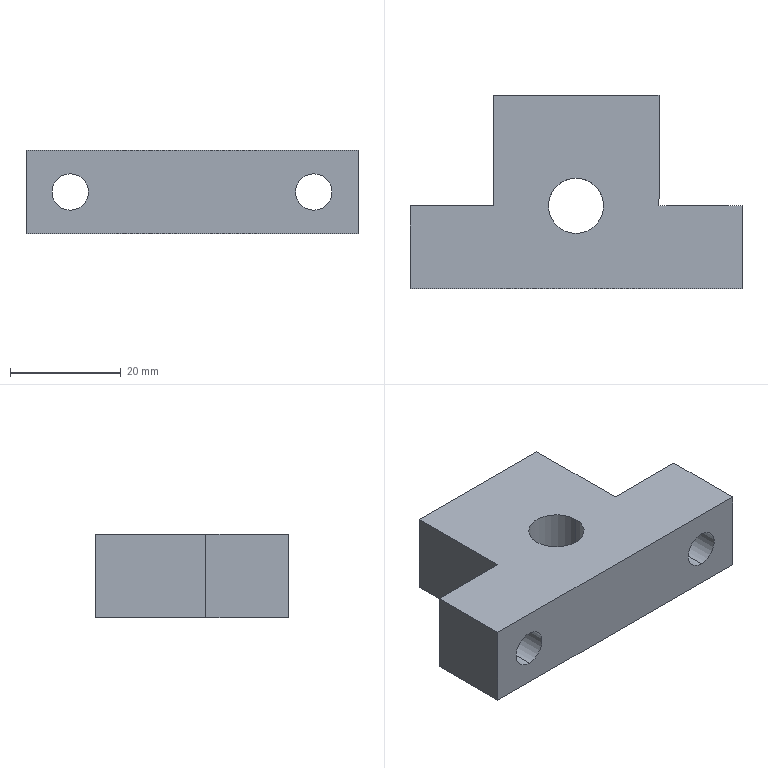Part | SolidWorks | features 3DProfileFeature 1, Extrusion 1, HoleWzd 1, ICE 1 | 1 solid | 22 faces | box 60 x 35 x 15 mm | volume 19468 mm3 | plane 12 | cylinder 10 | commonest cylinder face diameters 6.6 x4 11 x4 10 x2
STEP:
#1=CARTESIAN_POINT('',(8.,8.2,2.));
#2=VERTEX_POINT('',#1);
#3=CARTESIAN_POINT('',(8.,8.2,13.));
#4=VERTEX_POINT('',#3);
#5=CARTESIAN_POINT('',(8.,8.2,7.5));
#6=DIRECTION('',(0.,1.,0.));
#7=DIRECTION('',(0.,0.,1.));
#8=AXIS2_PLACEMENT_3D('',#5,#6,#7);
#9=CIRCLE('',#8,5.5);
#10=EDGE_CURVE('',#2,#4,#9,.T.);
#11=ORIENTED_EDGE('',*,*,#10,.F.);
#12=CARTESIAN_POINT('',(8.,15.,2.));
#13=VERTEX_POINT('',#12);
#14=CARTESIAN_POINT('',(8.,15.,2.));
#15=DIRECTION('',(0.,1.,0.));
#16=VECTOR('',#15,1000.);
#17=LINE('',#14,#16);
#18=EDGE_CURVE('',#2,#13,#17,.T.);
#19=ORIENTED_EDGE('',*,*,#18,.T.);
#20=CARTESIAN_POINT('',(8.,15.,13.));
#21=VERTEX_POINT('',#20);
#22=CARTESIAN_POINT('',(8.,15.,7.5));
#23=DIRECTION('',(0.,1.,0.));
#24=DIRECTION('',(0.,0.,1.));
#25=AXIS2_PLACEMENT_3D('',#22,#23,#24);
#26=CIRCLE('',#25,5.5);
#27=EDGE_CURVE('',#13,#21,#26,.T.);
#28=ORIENTED_EDGE('',*,*,#27,.T.);
#29=CARTESIAN_POINT('',(8.,15.,13.));
#30=DIRECTION('',(0.,1.,0.));
#31=VECTOR('',#30,1000.);
#32=LINE('',#29,#31);
#33=EDGE_CURVE('',#4,#21,#32,.T.);
#34=ORIENTED_EDGE('',*,*,#33,.F.);
#35=EDGE_LOOP('',(#11,#19,#28,#34));
#36=FACE_OUTER_BOUND('',#35,.T.);
#37=CARTESIAN_POINT('',(8.,15.,7.5));
#38=DIRECTION('',(0.,1.,0.));
#39=DIRECTION('',(0.,0.,1.));
#40=AXIS2_PLACEMENT_3D('',#37,#38,#39);
#41=CYLINDRICAL_SURFACE('',#40,5.5);
#42=ADVANCED_FACE('',(#36),#41,.F.);
#43=CARTESIAN_POINT('',(8.,0.,4.2));
#44=VERTEX_POINT('',#43);
#45=CARTESIAN_POINT('',(8.,0.,10.8));
#46=VERTEX_POINT('',#45);
#47=CARTESIAN_POINT('',(8.,0.,7.5));
#48=DIRECTION('',(0.,1.,0.));
#49=DIRECTION('',(0.,0.,1.));
#50=AXIS2_PLACEMENT_3D('',#47,#48,#49);
#51=CIRCLE('',#50,3.3);
#52=EDGE_CURVE('',#44,#46,#51,.T.);
#53=ORIENTED_EDGE('',*,*,#52,.F.);
#54=CARTESIAN_POINT('',(8.,8.2,4.2));
#55=VERTEX_POINT('',#54);
#56=CARTESIAN_POINT('',(8.,15.,4.2));
#57=DIRECTION('',(0.,1.,0.));
#58=VECTOR('',#57,1000.);
#59=LINE('',#56,#58);
#60=EDGE_CURVE('',#44,#55,#59,.T.);
#61=ORIENTED_EDGE('',*,*,#60,.T.);
#62=CARTESIAN_POINT('',(8.,8.2,10.8));
#63=VERTEX_POINT('',#62);
#64=CARTESIAN_POINT('',(8.,8.2,7.5));
#65=DIRECTION('',(0.,1.,0.));
#66=DIRECTION('',(0.,0.,1.));
#67=AXIS2_PLACEMENT_3D('',#64,#65,#66);
#68=CIRCLE('',#67,3.3);
#69=EDGE_CURVE('',#55,#63,#68,.T.);
#70=ORIENTED_EDGE('',*,*,#69,.T.);
#71=CARTESIAN_POINT('',(8.,15.,10.8));
#72=DIRECTION('',(0.,1.,0.));
#73=VECTOR('',#72,1000.);
#74=LINE('',#71,#73);
#75=EDGE_CURVE('',#46,#63,#74,.T.);
#76=ORIENTED_EDGE('',*,*,#75,.F.);
#77=EDGE_LOOP('',(#53,#61,#70,#76));
#78=FACE_OUTER_BOUND('',#77,.T.);
#79=CARTESIAN_POINT('',(8.,15.,7.5));
#80=DIRECTION('',(0.,1.,0.));
#81=DIRECTION('',(0.,0.,1.));
#82=AXIS2_PLACEMENT_3D('',#79,#80,#81);
#83=CYLINDRICAL_SURFACE('',#82,3.3);
#84=ADVANCED_FACE('',(#78),#83,.F.);
#85=CARTESIAN_POINT('',(52.,8.2,2.));
#86=VERTEX_POINT('',#85);
#87=CARTESIAN_POINT('',(52.,8.2,13.));
#88=VERTEX_POINT('',#87);
#89=CARTESIAN_POINT('',(52.,8.2,7.5));
#90=DIRECTION('',(0.,1.,0.));
#91=DIRECTION('',(0.,0.,1.));
#92=AXIS2_PLACEMENT_3D('',#89,#90,#91);
#93=CIRCLE('',#92,5.5);
#94=EDGE_CURVE('',#86,#88,#93,.T.);
#95=ORIENTED_EDGE('',*,*,#94,.F.);
#96=CARTESIAN_POINT('',(52.,15.,2.));
#97=VERTEX_POINT('',#96);
#98=CARTESIAN_POINT('',(52.,15.,2.));
#99=DIRECTION('',(0.,1.,0.));
#100=VECTOR('',#99,1000.);
#101=LINE('',#98,#100);
#102=EDGE_CURVE('',#86,#97,#101,.T.);
#103=ORIENTED_EDGE('',*,*,#102,.T.);
#104=CARTESIAN_POINT('',(52.,15.,13.));
#105=VERTEX_POINT('',#104);
#106=CARTESIAN_POINT('',(52.,15.,7.5));
#107=DIRECTION('',(0.,1.,0.));
#108=DIRECTION('',(0.,0.,1.));
#109=AXIS2_PLACEMENT_3D('',#106,#107,#108);
#110=CIRCLE('',#109,5.5);
#111=EDGE_CURVE('',#97,#105,#110,.T.);
#112=ORIENTED_EDGE('',*,*,#111,.T.);
#113=CARTESIAN_POINT('',(52.,15.,13.));
#114=DIRECTION('',(0.,1.,0.));
#115=VECTOR('',#114,1000.);
#116=LINE('',#113,#115);
#117=EDGE_CURVE('',#88,#105,#116,.T.);
#118=ORIENTED_EDGE('',*,*,#117,.F.);
#119=EDGE_LOOP('',(#95,#103,#112,#118));
#120=FACE_OUTER_BOUND('',#119,.T.);
#121=CARTESIAN_POINT('',(52.,15.,7.5));
#122=DIRECTION('',(0.,1.,0.));
#123=DIRECTION('',(0.,0.,1.));
#124=AXIS2_PLACEMENT_3D('',#121,#122,#123);
#125=CYLINDRICAL_SURFACE('',#124,5.5);
#126=ADVANCED_FACE('',(#120),#125,.F.);
#127=CARTESIAN_POINT('',(52.,0.,4.2));
#128=VERTEX_POINT('',#127);
#129=CARTESIAN_POINT('',(52.,0.,10.8));
#130=VERTEX_POINT('',#129);
#131=CARTESIAN_POINT('',(52.,0.,7.5));
#132=DIRECTION('',(0.,1.,0.));
#133=DIRECTION('',(0.,0.,1.));
#134=AXIS2_PLACEMENT_3D('',#131,#132,#133);
#135=CIRCLE('',#134,3.3);
#136=EDGE_CURVE('',#128,#130,#135,.T.);
#137=ORIENTED_EDGE('',*,*,#136,.F.);
#138=CARTESIAN_POINT('',(52.,8.2,4.2));
#139=VERTEX_POINT('',#138);
#140=CARTESIAN_POINT('',(52.,15.,4.2));
#141=DIRECTION('',(0.,1.,0.));
#142=VECTOR('',#141,1000.);
#143=LINE('',#140,#142);
#144=EDGE_CURVE('',#128,#139,#143,.T.);
#145=ORIENTED_EDGE('',*,*,#144,.T.);
#146=CARTESIAN_POINT('',(52.,8.2,10.8));
#147=VERTEX_POINT('',#146);
#148=CARTESIAN_POINT('',(52.,8.2,7.5));
#149=DIRECTION('',(0.,1.,0.));
#150=DIRECTION('',(0.,0.,1.));
#151=AXIS2_PLACEMENT_3D('',#148,#149,#150);
#152=CIRCLE('',#151,3.3);
#153=EDGE_CURVE('',#139,#147,#152,.T.);
#154=ORIENTED_EDGE('',*,*,#153,.T.);
#155=CARTESIAN_POINT('',(52.,15.,10.8));
#156=DIRECTION('',(0.,1.,0.));
#157=VECTOR('',#156,1000.);
#158=LINE('',#155,#157);
#159=EDGE_CURVE('',#130,#147,#158,.T.);
#160=ORIENTED_EDGE('',*,*,#159,.F.);
#161=EDGE_LOOP('',(#137,#145,#154,#160));
#162=FACE_OUTER_BOUND('',#161,.T.);
#163=CARTESIAN_POINT('',(52.,15.,7.5));
#164=DIRECTION('',(0.,1.,0.));
#165=DIRECTION('',(0.,0.,1.));
#166=AXIS2_PLACEMENT_3D('',#163,#164,#165);
#167=CYLINDRICAL_SURFACE('',#166,3.3);
#168=ADVANCED_FACE('',(#162),#167,.F.);
#169=CARTESIAN_POINT('',(25.,15.,0.));
#170=VERTEX_POINT('',#169);
#171=CARTESIAN_POINT('',(35.,15.,0.));
#172=VERTEX_POINT('',#171);
#173=CARTESIAN_POINT('',(30.,15.,0.));
#174=DIRECTION('',(0.,0.,1.));
#175=DIRECTION('',(1.,0.,0.));
#176=AXIS2_PLACEMENT_3D('',#173,#174,#175);
#177=CIRCLE('',#176,5.);
#178=EDGE_CURVE('',#170,#172,#177,.T.);
#179=ORIENTED_EDGE('',*,*,#178,.F.);
#180=CARTESIAN_POINT('',(25.,15.,15.));
#181=VERTEX_POINT('',#180);
#182=CARTESIAN_POINT('',(25.,15.,0.));
#183=DIRECTION('',(0.,0.,1.));
#184=VECTOR('',#183,1000.);
#185=LINE('',#182,#184);
#186=EDGE_CURVE('',#170,#181,#185,.T.);
#187=ORIENTED_EDGE('',*,*,#186,.T.);
#188=CARTESIAN_POINT('',(35.,15.,15.));
#189=VERTEX_POINT('',#188);
#190=CARTESIAN_POINT('',(30.,15.,15.));
#191=DIRECTION('',(0.,0.,1.));
#192=DIRECTION('',(1.,0.,0.));
#193=AXIS2_PLACEMENT_3D('',#190,#191,#192);
#194=CIRCLE('',#193,5.);
#195=EDGE_CURVE('',#181,#189,#194,.T.);
#196=ORIENTED_EDGE('',*,*,#195,.T.);
#197=CARTESIAN_POINT('',(35.,15.,0.));
#198=DIRECTION('',(0.,0.,1.));
#199=VECTOR('',#198,1000.);
#200=LINE('',#197,#199);
#201=EDGE_CURVE('',#172,#189,#200,.T.);
#202=ORIENTED_EDGE('',*,*,#201,.F.);
#203=EDGE_LOOP('',(#179,#187,#196,#202));
#204=FACE_OUTER_BOUND('',#203,.T.);
#205=CARTESIAN_POINT('',(30.,15.,0.));
#206=DIRECTION('',(0.,0.,1.));
#207=DIRECTION('',(1.,0.,0.));
#208=AXIS2_PLACEMENT_3D('',#205,#206,#207);
#209=CYLINDRICAL_SURFACE('',#208,5.);
#210=ADVANCED_FACE('',(#204),#209,.F.);
#211=CARTESIAN_POINT('',(8.,0.,7.5));
#212=DIRECTION('',(0.,1.,0.));
#213=DIRECTION('',(0.,0.,1.));
#214=AXIS2_PLACEMENT_3D('',#211,#212,#213);
#215=CIRCLE('',#214,3.3);
#216=EDGE_CURVE('',#46,#44,#215,.T.);
#217=ORIENTED_EDGE('',*,*,#216,.T.);
#218=ORIENTED_EDGE('',*,*,#52,.T.);
#219=EDGE_LOOP('',(#217,#218));
#220=FACE_BOUND('',#219,.T.);
#221=CARTESIAN_POINT('',(52.,0.,7.5));
#222=DIRECTION('',(0.,1.,0.));
#223=DIRECTION('',(0.,0.,1.));
#224=AXIS2_PLACEMENT_3D('',#221,#222,#223);
#225=CIRCLE('',#224,3.3);
#226=EDGE_CURVE('',#130,#128,#225,.T.);
#227=ORIENTED_EDGE('',*,*,#226,.T.);
#228=ORIENTED_EDGE('',*,*,#136,.T.);
#229=EDGE_LOOP('',(#227,#228));
#230=FACE_BOUND('',#229,.T.);
#231=CARTESIAN_POINT('',(0.,0.,0.));
#232=VERTEX_POINT('',#231);
#233=CARTESIAN_POINT('',(60.,0.,0.));
#234=VERTEX_POINT('',#233);
#235=CARTESIAN_POINT('',(60.,0.,0.));
#236=DIRECTION('',(1.,0.,0.));
#237=VECTOR('',#236,1000.);
#238=LINE('',#235,#237);
#239=EDGE_CURVE('',#232,#234,#238,.T.);
#240=ORIENTED_EDGE('',*,*,#239,.T.);
#241=CARTESIAN_POINT('',(60.,0.,15.));
#242=VERTEX_POINT('',#241);
#243=CARTESIAN_POINT('',(60.,0.,15.));
#244=DIRECTION('',(0.,0.,-1.));
#245=VECTOR('',#244,1000.);
#246=LINE('',#243,#245);
#247=EDGE_CURVE('',#242,#234,#246,.T.);
#248=ORIENTED_EDGE('',*,*,#247,.F.);
#249=CARTESIAN_POINT('',(0.,0.,15.));
#250=VERTEX_POINT('',#249);
#251=CARTESIAN_POINT('',(60.,0.,15.));
#252=DIRECTION('',(1.,0.,0.));
#253=VECTOR('',#252,1000.);
#254=LINE('',#251,#253);
#255=EDGE_CURVE('',#250,#242,#254,.T.);
#256=ORIENTED_EDGE('',*,*,#255,.F.);
#257=CARTESIAN_POINT('',(0.,0.,15.));
#258=DIRECTION('',(0.,0.,-1.));
#259=VECTOR('',#258,1000.);
#260=LINE('',#257,#259);
#261=EDGE_CURVE('',#250,#232,#260,.T.);
#262=ORIENTED_EDGE('',*,*,#261,.T.);
#263=EDGE_LOOP('',(#240,#248,#256,#262));
#264=FACE_OUTER_BOUND('',#263,.T.);
#265=CARTESIAN_POINT('',(60.,0.,15.));
#266=DIRECTION('',(0.,1.,0.));
#267=DIRECTION('',(-1.,0.,0.));
#268=AXIS2_PLACEMENT_3D('',#265,#266,#267);
#269=PLANE('',#268);
#270=ADVANCED_FACE('',(#220,#230,#264),#269,.F.);
#271=CARTESIAN_POINT('',(60.,15.,0.));
#272=VERTEX_POINT('',#271);
#273=CARTESIAN_POINT('',(60.,0.,0.));
#274=DIRECTION('',(0.,1.,0.));
#275=VECTOR('',#274,1000.);
#276=LINE('',#273,#275);
#277=EDGE_CURVE('',#234,#272,#276,.T.);
#278=ORIENTED_EDGE('',*,*,#277,.T.);
#279=CARTESIAN_POINT('',(60.,15.,15.));
#280=VERTEX_POINT('',#279);
#281=CARTESIAN_POINT('',(60.,15.,15.));
#282=DIRECTION('',(0.,0.,-1.));
#283=VECTOR('',#282,1000.);
#284=LINE('',#281,#283);
#285=EDGE_CURVE('',#280,#272,#284,.T.);
#286=ORIENTED_EDGE('',*,*,#285,.F.);
#287=CARTESIAN_POINT('',(60.,0.,15.));
#288=DIRECTION('',(0.,1.,0.));
#289=VECTOR('',#288,1000.);
#290=LINE('',#287,#289);
#291=EDGE_CURVE('',#242,#280,#290,.T.);
#292=ORIENTED_EDGE('',*,*,#291,.F.);
#293=ORIENTED_EDGE('',*,*,#247,.T.);
#294=EDGE_LOOP('',(#278,#286,#292,#293));
#295=FACE_OUTER_BOUND('',#294,.T.);
#296=CARTESIAN_POINT('',(60.,0.,15.));
#297=DIRECTION('',(-1.,0.,0.));
#298=DIRECTION('',(0.,0.,1.));
#299=AXIS2_PLACEMENT_3D('',#296,#297,#298);
#300=PLANE('',#299);
#301=ADVANCED_FACE('',(#295),#300,.F.);
#302=CARTESIAN_POINT('',(52.,15.,7.5));
#303=DIRECTION('',(0.,1.,0.));
#304=DIRECTION('',(0.,0.,1.));
#305=AXIS2_PLACEMENT_3D('',#302,#303,#304);
#306=CIRCLE('',#305,5.5);
#307=EDGE_CURVE('',#105,#97,#306,.T.);
#308=ORIENTED_EDGE('',*,*,#307,.F.);
#309=ORIENTED_EDGE('',*,*,#111,.F.);
#310=EDGE_LOOP('',(#308,#309));
#311=FACE_BOUND('',#310,.T.);
#312=CARTESIAN_POINT('',(45.,15.,0.));
#313=VERTEX_POINT('',#312);
#314=CARTESIAN_POINT('',(60.,15.,0.));
#315=DIRECTION('',(-1.,0.,0.));
#316=VECTOR('',#315,1000.);
#317=LINE('',#314,#316);
#318=EDGE_CURVE('',#272,#313,#317,.T.);
#319=ORIENTED_EDGE('',*,*,#318,.T.);
#320=CARTESIAN_POINT('',(45.,15.,15.));
#321=VERTEX_POINT('',#320);
#322=CARTESIAN_POINT('',(45.,15.,15.));
#323=DIRECTION('',(0.,0.,-1.));
#324=VECTOR('',#323,1000.);
#325=LINE('',#322,#324);
#326=EDGE_CURVE('',#321,#313,#325,.T.);
#327=ORIENTED_EDGE('',*,*,#326,.F.);
#328=CARTESIAN_POINT('',(60.,15.,15.));
#329=DIRECTION('',(-1.,0.,0.));
#330=VECTOR('',#329,1000.);
#331=LINE('',#328,#330);
#332=EDGE_CURVE('',#280,#321,#331,.T.);
#333=ORIENTED_EDGE('',*,*,#332,.F.);
#334=ORIENTED_EDGE('',*,*,#285,.T.);
#335=EDGE_LOOP('',(#319,#327,#333,#334));
#336=FACE_OUTER_BOUND('',#335,.T.);
#337=CARTESIAN_POINT('',(60.,15.,15.));
#338=DIRECTION('',(0.,-1.,0.));
#339=DIRECTION('',(0.,0.,-1.));
#340=AXIS2_PLACEMENT_3D('',#337,#338,#339);
#341=PLANE('',#340);
#342=ADVANCED_FACE('',(#311,#336),#341,.F.);
#343=CARTESIAN_POINT('',(45.,35.,0.));
#344=VERTEX_POINT('',#343);
#345=CARTESIAN_POINT('',(45.,15.,0.));
#346=DIRECTION('',(0.,1.,0.));
#347=VECTOR('',#346,1000.);
#348=LINE('',#345,#347);
#349=EDGE_CURVE('',#313,#344,#348,.T.);
#350=ORIENTED_EDGE('',*,*,#349,.T.);
#351=CARTESIAN_POINT('',(45.,35.,15.));
#352=VERTEX_POINT('',#351);
#353=CARTESIAN_POINT('',(45.,35.,15.));
#354=DIRECTION('',(0.,0.,-1.));
#355=VECTOR('',#354,1000.);
#356=LINE('',#353,#355);
#357=EDGE_CURVE('',#352,#344,#356,.T.);
#358=ORIENTED_EDGE('',*,*,#357,.F.);
#359=CARTESIAN_POINT('',(45.,15.,15.));
#360=DIRECTION('',(0.,1.,0.));
#361=VECTOR('',#360,1000.);
#362=LINE('',#359,#361);
#363=EDGE_CURVE('',#321,#352,#362,.T.);
#364=ORIENTED_EDGE('',*,*,#363,.F.);
#365=ORIENTED_EDGE('',*,*,#326,.T.);
#366=EDGE_LOOP('',(#350,#358,#364,#365));
#367=FACE_OUTER_BOUND('',#366,.T.);
#368=CARTESIAN_POINT('',(45.,15.,15.));
#369=DIRECTION('',(-1.,0.,0.));
#370=DIRECTION('',(0.,0.,1.));
#371=AXIS2_PLACEMENT_3D('',#368,#369,#370);
#372=PLANE('',#371);
#373=ADVANCED_FACE('',(#367),#372,.F.);
#374=CARTESIAN_POINT('',(15.,35.,0.));
#375=VERTEX_POINT('',#374);
#376=CARTESIAN_POINT('',(15.,35.,0.));
#377=DIRECTION('',(-1.,0.,0.));
#378=VECTOR('',#377,1000.);
#379=LINE('',#376,#378);
#380=EDGE_CURVE('',#344,#375,#379,.T.);
#381=ORIENTED_EDGE('',*,*,#380,.T.);
#382=CARTESIAN_POINT('',(15.,35.,15.));
#383=VERTEX_POINT('',#382);
#384=CARTESIAN_POINT('',(15.,35.,15.));
#385=DIRECTION('',(0.,0.,-1.));
#386=VECTOR('',#385,1000.);
#387=LINE('',#384,#386);
#388=EDGE_CURVE('',#383,#375,#387,.T.);
#389=ORIENTED_EDGE('',*,*,#388,.F.);
#390=CARTESIAN_POINT('',(15.,35.,15.));
#391=DIRECTION('',(-1.,0.,0.));
#392=VECTOR('',#391,1000.);
#393=LINE('',#390,#392);
#394=EDGE_CURVE('',#352,#383,#393,.T.);
#395=ORIENTED_EDGE('',*,*,#394,.F.);
#396=ORIENTED_EDGE('',*,*,#357,.T.);
#397=EDGE_LOOP('',(#381,#389,#395,#396));
#398=FACE_OUTER_BOUND('',#397,.T.);
#399=CARTESIAN_POINT('',(15.,35.,15.));
#400=DIRECTION('',(0.,-1.,0.));
#401=DIRECTION('',(0.,0.,-1.));
#402=AXIS2_PLACEMENT_3D('',#399,#400,#401);
#403=PLANE('',#402);
#404=ADVANCED_FACE('',(#398),#403,.F.);
#405=CARTESIAN_POINT('',(15.,15.,0.));
#406=VERTEX_POINT('',#405);
#407=CARTESIAN_POINT('',(15.,15.,0.));
#408=DIRECTION('',(0.,-1.,0.));
#409=VECTOR('',#408,1000.);
#410=LINE('',#407,#409);
#411=EDGE_CURVE('',#375,#406,#410,.T.);
#412=ORIENTED_EDGE('',*,*,#411,.T.);
#413=CARTESIAN_POINT('',(15.,15.,15.));
#414=VERTEX_POINT('',#413);
#415=CARTESIAN_POINT('',(15.,15.,15.));
#416=DIRECTION('',(0.,0.,-1.));
#417=VECTOR('',#416,1000.);
#418=LINE('',#415,#417);
#419=EDGE_CURVE('',#414,#406,#418,.T.);
#420=ORIENTED_EDGE('',*,*,#419,.F.);
#421=CARTESIAN_POINT('',(15.,15.,15.));
#422=DIRECTION('',(0.,-1.,0.));
#423=VECTOR('',#422,1000.);
#424=LINE('',#421,#423);
#425=EDGE_CURVE('',#383,#414,#424,.T.);
#426=ORIENTED_EDGE('',*,*,#425,.F.);
#427=ORIENTED_EDGE('',*,*,#388,.T.);
#428=EDGE_LOOP('',(#412,#420,#426,#427));
#429=FACE_OUTER_BOUND('',#428,.T.);
#430=CARTESIAN_POINT('',(15.,15.,15.));
#431=DIRECTION('',(1.,0.,0.));
#432=DIRECTION('',(0.,0.,-1.));
#433=AXIS2_PLACEMENT_3D('',#430,#431,#432);
#434=PLANE('',#433);
#435=ADVANCED_FACE('',(#429),#434,.F.);
#436=CARTESIAN_POINT('',(8.,15.,7.5));
#437=DIRECTION('',(0.,1.,0.));
#438=DIRECTION('',(0.,0.,1.));
#439=AXIS2_PLACEMENT_3D('',#436,#437,#438);
#440=CIRCLE('',#439,5.5);
#441=EDGE_CURVE('',#21,#13,#440,.T.);
#442=ORIENTED_EDGE('',*,*,#441,.F.);
#443=ORIENTED_EDGE('',*,*,#27,.F.);
#444=EDGE_LOOP('',(#442,#443));
#445=FACE_BOUND('',#444,.T.);
#446=CARTESIAN_POINT('',(0.,15.,0.));
#447=VERTEX_POINT('',#446);
#448=CARTESIAN_POINT('',(0.,15.,0.));
#449=DIRECTION('',(-1.,0.,0.));
#450=VECTOR('',#449,1000.);
#451=LINE('',#448,#450);
#452=EDGE_CURVE('',#406,#447,#451,.T.);
#453=ORIENTED_EDGE('',*,*,#452,.T.);
#454=CARTESIAN_POINT('',(0.,15.,15.));
#455=VERTEX_POINT('',#454);
#456=CARTESIAN_POINT('',(0.,15.,15.));
#457=DIRECTION('',(0.,0.,-1.));
#458=VECTOR('',#457,1000.);
#459=LINE('',#456,#458);
#460=EDGE_CURVE('',#455,#447,#459,.T.);
#461=ORIENTED_EDGE('',*,*,#460,.F.);
#462=CARTESIAN_POINT('',(0.,15.,15.));
#463=DIRECTION('',(-1.,0.,0.));
#464=VECTOR('',#463,1000.);
#465=LINE('',#462,#464);
#466=EDGE_CURVE('',#414,#455,#465,.T.);
#467=ORIENTED_EDGE('',*,*,#466,.F.);
#468=ORIENTED_EDGE('',*,*,#419,.T.);
#469=EDGE_LOOP('',(#453,#461,#467,#468));
#470=FACE_OUTER_BOUND('',#469,.T.);
#471=CARTESIAN_POINT('',(0.,15.,15.));
#472=DIRECTION('',(0.,-1.,0.));
#473=DIRECTION('',(0.,0.,-1.));
#474=AXIS2_PLACEMENT_3D('',#471,#472,#473);
#475=PLANE('',#474);
#476=ADVANCED_FACE('',(#445,#470),#475,.F.);
#477=CARTESIAN_POINT('',(0.,0.,0.));
#478=DIRECTION('',(0.,-1.,0.));
#479=VECTOR('',#478,1000.);
#480=LINE('',#477,#479);
#481=EDGE_CURVE('',#447,#232,#480,.T.);
#482=ORIENTED_EDGE('',*,*,#481,.T.);
#483=ORIENTED_EDGE('',*,*,#261,.F.);
#484=CARTESIAN_POINT('',(0.,0.,15.));
#485=DIRECTION('',(0.,-1.,0.));
#486=VECTOR('',#485,1000.);
#487=LINE('',#484,#486);
#488=EDGE_CURVE('',#455,#250,#487,.T.);
#489=ORIENTED_EDGE('',*,*,#488,.F.);
#490=ORIENTED_EDGE('',*,*,#460,.T.);
#491=EDGE_LOOP('',(#482,#483,#489,#490));
#492=FACE_OUTER_BOUND('',#491,.T.);
#493=CARTESIAN_POINT('',(0.,0.,15.));
#494=DIRECTION('',(1.,0.,0.));
#495=DIRECTION('',(0.,0.,-1.));
#496=AXIS2_PLACEMENT_3D('',#493,#494,#495);
#497=PLANE('',#496);
#498=ADVANCED_FACE('',(#492),#497,.F.);
#499=CARTESIAN_POINT('',(30.,15.,15.));
#500=DIRECTION('',(0.,0.,1.));
#501=DIRECTION('',(1.,0.,0.));
#502=AXIS2_PLACEMENT_3D('',#499,#500,#501);
#503=CIRCLE('',#502,5.);
#504=EDGE_CURVE('',#189,#181,#503,.T.);
#505=ORIENTED_EDGE('',*,*,#504,.F.);
#506=ORIENTED_EDGE('',*,*,#195,.F.);
#507=EDGE_LOOP('',(#505,#506));
#508=FACE_BOUND('',#507,.T.);
#509=ORIENTED_EDGE('',*,*,#255,.T.);
#510=ORIENTED_EDGE('',*,*,#291,.T.);
#511=ORIENTED_EDGE('',*,*,#332,.T.);
#512=ORIENTED_EDGE('',*,*,#363,.T.);
#513=ORIENTED_EDGE('',*,*,#394,.T.);
#514=ORIENTED_EDGE('',*,*,#425,.T.);
#515=ORIENTED_EDGE('',*,*,#466,.T.);
#516=ORIENTED_EDGE('',*,*,#488,.T.);
#517=EDGE_LOOP('',(#509,#510,#511,#512,#513,#514,#515,#516));
#518=FACE_OUTER_BOUND('',#517,.T.);
#519=CARTESIAN_POINT('',(0.,0.,15.));
#520=DIRECTION('',(0.,0.,-1.));
#521=DIRECTION('',(-1.,0.,0.));
#522=AXIS2_PLACEMENT_3D('',#519,#520,#521);
#523=PLANE('',#522);
#524=ADVANCED_FACE('',(#508,#518),#523,.F.);
#525=CARTESIAN_POINT('',(30.,15.,0.));
#526=DIRECTION('',(0.,0.,1.));
#527=DIRECTION('',(1.,0.,0.));
#528=AXIS2_PLACEMENT_3D('',#525,#526,#527);
#529=CIRCLE('',#528,5.);
#530=EDGE_CURVE('',#172,#170,#529,.T.);
#531=ORIENTED_EDGE('',*,*,#530,.T.);
#532=ORIENTED_EDGE('',*,*,#178,.T.);
#533=EDGE_LOOP('',(#531,#532));
#534=FACE_BOUND('',#533,.T.);
#535=ORIENTED_EDGE('',*,*,#239,.F.);
#536=ORIENTED_EDGE('',*,*,#481,.F.);
#537=ORIENTED_EDGE('',*,*,#452,.F.);
#538=ORIENTED_EDGE('',*,*,#411,.F.);
#539=ORIENTED_EDGE('',*,*,#380,.F.);
#540=ORIENTED_EDGE('',*,*,#349,.F.);
#541=ORIENTED_EDGE('',*,*,#318,.F.);
#542=ORIENTED_EDGE('',*,*,#277,.F.);
#543=EDGE_LOOP('',(#535,#536,#537,#538,#539,#540,#541,#542));
#544=FACE_OUTER_BOUND('',#543,.T.);
#545=CARTESIAN_POINT('',(0.,0.,0.));
#546=DIRECTION('',(0.,0.,-1.));
#547=DIRECTION('',(-1.,0.,0.));
#548=AXIS2_PLACEMENT_3D('',#545,#546,#547);
#549=PLANE('',#548);
#550=ADVANCED_FACE('',(#534,#544),#549,.T.);
#551=ORIENTED_EDGE('',*,*,#186,.F.);
#552=ORIENTED_EDGE('',*,*,#530,.F.);
#553=ORIENTED_EDGE('',*,*,#201,.T.);
#554=ORIENTED_EDGE('',*,*,#504,.T.);
#555=EDGE_LOOP('',(#551,#552,#553,#554));
#556=FACE_OUTER_BOUND('',#555,.T.);
#557=CARTESIAN_POINT('',(30.,15.,0.));
#558=DIRECTION('',(0.,0.,1.));
#559=DIRECTION('',(1.,0.,0.));
#560=AXIS2_PLACEMENT_3D('',#557,#558,#559);
#561=CYLINDRICAL_SURFACE('',#560,5.);
#562=ADVANCED_FACE('',(#556),#561,.F.);
#563=ORIENTED_EDGE('',*,*,#144,.F.);
#564=ORIENTED_EDGE('',*,*,#226,.F.);
#565=ORIENTED_EDGE('',*,*,#159,.T.);
#566=CARTESIAN_POINT('',(52.,8.2,7.5));
#567=DIRECTION('',(0.,1.,0.));
#568=DIRECTION('',(0.,0.,1.));
#569=AXIS2_PLACEMENT_3D('',#566,#567,#568);
#570=CIRCLE('',#569,3.3);
#571=EDGE_CURVE('',#147,#139,#570,.T.);
#572=ORIENTED_EDGE('',*,*,#571,.T.);
#573=EDGE_LOOP('',(#563,#564,#565,#572));
#574=FACE_OUTER_BOUND('',#573,.T.);
#575=CARTESIAN_POINT('',(52.,15.,7.5));
#576=DIRECTION('',(0.,1.,0.));
#577=DIRECTION('',(0.,0.,1.));
#578=AXIS2_PLACEMENT_3D('',#575,#576,#577);
#579=CYLINDRICAL_SURFACE('',#578,3.3);
#580=ADVANCED_FACE('',(#574),#579,.F.);
#581=ORIENTED_EDGE('',*,*,#571,.F.);
#582=ORIENTED_EDGE('',*,*,#153,.F.);
#583=EDGE_LOOP('',(#581,#582));
#584=FACE_BOUND('',#583,.T.);
#585=CARTESIAN_POINT('',(52.,8.2,7.5));
#586=DIRECTION('',(0.,1.,0.));
#587=DIRECTION('',(0.,0.,1.));
#588=AXIS2_PLACEMENT_3D('',#585,#586,#587);
#589=CIRCLE('',#588,5.5);
#590=EDGE_CURVE('',#88,#86,#589,.T.);
#591=ORIENTED_EDGE('',*,*,#590,.T.);
#592=ORIENTED_EDGE('',*,*,#94,.T.);
#593=EDGE_LOOP('',(#591,#592));
#594=FACE_OUTER_BOUND('',#593,.T.);
#595=CARTESIAN_POINT('',(55.3,8.2,7.5));
#596=DIRECTION('',(0.,-1.,0.));
#597=DIRECTION('',(0.,0.,-1.));
#598=AXIS2_PLACEMENT_3D('',#595,#596,#597);
#599=PLANE('',#598);
#600=ADVANCED_FACE('',(#584,#594),#599,.F.);
#601=ORIENTED_EDGE('',*,*,#102,.F.);
#602=ORIENTED_EDGE('',*,*,#590,.F.);
#603=ORIENTED_EDGE('',*,*,#117,.T.);
#604=ORIENTED_EDGE('',*,*,#307,.T.);
#605=EDGE_LOOP('',(#601,#602,#603,#604));
#606=FACE_OUTER_BOUND('',#605,.T.);
#607=CARTESIAN_POINT('',(52.,15.,7.5));
#608=DIRECTION('',(0.,1.,0.));
#609=DIRECTION('',(0.,0.,1.));
#610=AXIS2_PLACEMENT_3D('',#607,#608,#609);
#611=CYLINDRICAL_SURFACE('',#610,5.5);
#612=ADVANCED_FACE('',(#606),#611,.F.);
#613=ORIENTED_EDGE('',*,*,#60,.F.);
#614=ORIENTED_EDGE('',*,*,#216,.F.);
#615=ORIENTED_EDGE('',*,*,#75,.T.);
#616=CARTESIAN_POINT('',(8.,8.2,7.5));
#617=DIRECTION('',(0.,1.,0.));
#618=DIRECTION('',(0.,0.,1.));
#619=AXIS2_PLACEMENT_3D('',#616,#617,#618);
#620=CIRCLE('',#619,3.3);
#621=EDGE_CURVE('',#63,#55,#620,.T.);
#622=ORIENTED_EDGE('',*,*,#621,.T.);
#623=EDGE_LOOP('',(#613,#614,#615,#622));
#624=FACE_OUTER_BOUND('',#623,.T.);
#625=CARTESIAN_POINT('',(8.,15.,7.5));
#626=DIRECTION('',(0.,1.,0.));
#627=DIRECTION('',(0.,0.,1.));
#628=AXIS2_PLACEMENT_3D('',#625,#626,#627);
#629=CYLINDRICAL_SURFACE('',#628,3.3);
#630=ADVANCED_FACE('',(#624),#629,.F.);
#631=ORIENTED_EDGE('',*,*,#621,.F.);
#632=ORIENTED_EDGE('',*,*,#69,.F.);
#633=EDGE_LOOP('',(#631,#632));
#634=FACE_BOUND('',#633,.T.);
#635=CARTESIAN_POINT('',(8.,8.2,7.5));
#636=DIRECTION('',(0.,1.,0.));
#637=DIRECTION('',(0.,0.,1.));
#638=AXIS2_PLACEMENT_3D('',#635,#636,#637);
#639=CIRCLE('',#638,5.5);
#640=EDGE_CURVE('',#4,#2,#639,.T.);
#641=ORIENTED_EDGE('',*,*,#640,.T.);
#642=ORIENTED_EDGE('',*,*,#10,.T.);
#643=EDGE_LOOP('',(#641,#642));
#644=FACE_OUTER_BOUND('',#643,.T.);
#645=CARTESIAN_POINT('',(11.3,8.2,7.5));
#646=DIRECTION('',(0.,-1.,0.));
#647=DIRECTION('',(0.,0.,-1.));
#648=AXIS2_PLACEMENT_3D('',#645,#646,#647);
#649=PLANE('',#648);
#650=ADVANCED_FACE('',(#634,#644),#649,.F.);
#651=ORIENTED_EDGE('',*,*,#18,.F.);
#652=ORIENTED_EDGE('',*,*,#640,.F.);
#653=ORIENTED_EDGE('',*,*,#33,.T.);
#654=ORIENTED_EDGE('',*,*,#441,.T.);
#655=EDGE_LOOP('',(#651,#652,#653,#654));
#656=FACE_OUTER_BOUND('',#655,.T.);
#657=CARTESIAN_POINT('',(8.,15.,7.5));
#658=DIRECTION('',(0.,1.,0.));
#659=DIRECTION('',(0.,0.,1.));
#660=AXIS2_PLACEMENT_3D('',#657,#658,#659);
#661=CYLINDRICAL_SURFACE('',#660,5.5);
#662=ADVANCED_FACE('',(#656),#661,.F.);
#663=CLOSED_SHELL('',(#42,#84,#126,#168,#210,#270,#301,#342,#373,#404,#435,#476,#498,#524,#550,#562,#580,#600,#612,#630,#650,#662));
#664=MANIFOLD_SOLID_BREP('',#663);
#665=CARTESIAN_POINT('',(0.,0.,0.));
#666=DIRECTION('',(0.,0.,1.));
#667=DIRECTION('',(1.,0.,0.));
#668=AXIS2_PLACEMENT_3D('',#665,#666,#667);
#669=(LENGTH_UNIT()NAMED_UNIT(*)SI_UNIT(.MILLI.,.METRE.));
#670=UNCERTAINTY_MEASURE_WITH_UNIT(LENGTH_MEASURE(0.00001),#669,'','');
#671=(NAMED_UNIT(*)PLANE_ANGLE_UNIT()SI_UNIT($,.RADIAN.));
#672=(NAMED_UNIT(*)SI_UNIT($,.STERADIAN.)SOLID_ANGLE_UNIT());
#673=(GEOMETRIC_REPRESENTATION_CONTEXT(3)GLOBAL_UNCERTAINTY_ASSIGNED_CONTEXT((#670))GLOBAL_UNIT_ASSIGNED_CONTEXT((#669,#671,#672))REPRESENTATION_CONTEXT('',''));
#674=ADVANCED_BREP_SHAPE_REPRESENTATION('',(#664,#668),#673);